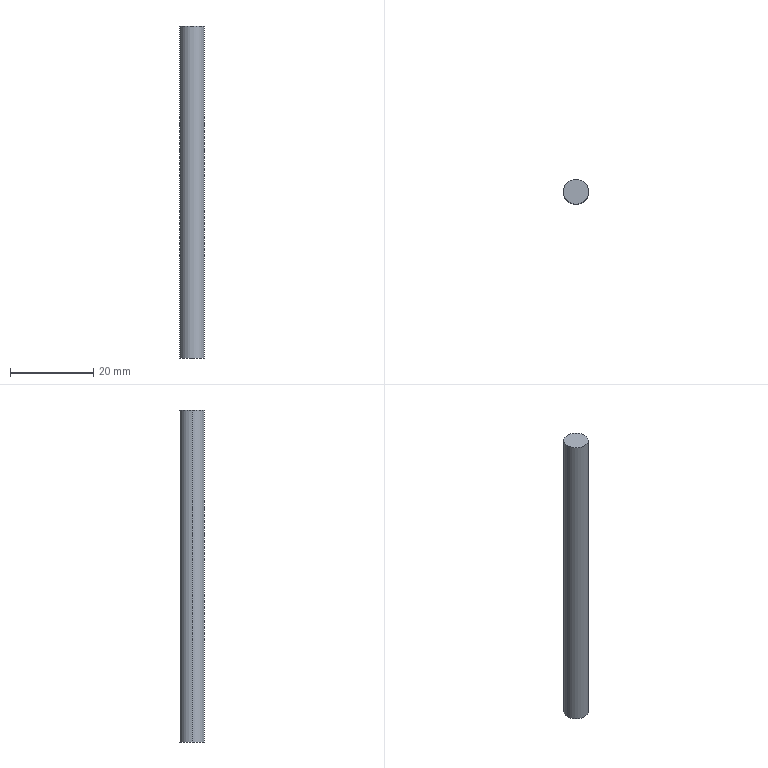Part | SolidWorks | features Extrusion 1 | 1 solid | 4 faces | box 6 x 6 x 80 mm | volume 2262 mm3 | cylinder 2 | plane 2 | commonest cylinder face diameters 6 x2
STEP:
#1=CARTESIAN_POINT('',(3.,0.,80.));
#2=VERTEX_POINT('',#1);
#3=CARTESIAN_POINT('',(-3.,0.,80.));
#4=VERTEX_POINT('',#3);
#5=CARTESIAN_POINT('',(0.,0.,80.));
#6=DIRECTION('',(0.,0.,1.));
#7=DIRECTION('',(1.,0.,0.));
#8=AXIS2_PLACEMENT_3D('',#5,#6,#7);
#9=CIRCLE('',#8,3.);
#10=EDGE_CURVE('',#2,#4,#9,.T.);
#11=ORIENTED_EDGE('',*,*,#10,.F.);
#12=CARTESIAN_POINT('',(3.,0.,0.));
#13=VERTEX_POINT('',#12);
#14=CARTESIAN_POINT('',(3.,0.,80.));
#15=DIRECTION('',(0.,0.,-1.));
#16=VECTOR('',#15,1000.);
#17=LINE('',#14,#16);
#18=EDGE_CURVE('',#2,#13,#17,.T.);
#19=ORIENTED_EDGE('',*,*,#18,.T.);
#20=CARTESIAN_POINT('',(-3.,0.,0.));
#21=VERTEX_POINT('',#20);
#22=CARTESIAN_POINT('',(0.,0.,0.));
#23=DIRECTION('',(0.,0.,1.));
#24=DIRECTION('',(1.,0.,0.));
#25=AXIS2_PLACEMENT_3D('',#22,#23,#24);
#26=CIRCLE('',#25,3.);
#27=EDGE_CURVE('',#13,#21,#26,.T.);
#28=ORIENTED_EDGE('',*,*,#27,.T.);
#29=CARTESIAN_POINT('',(-3.,0.,80.));
#30=DIRECTION('',(0.,0.,-1.));
#31=VECTOR('',#30,1000.);
#32=LINE('',#29,#31);
#33=EDGE_CURVE('',#4,#21,#32,.T.);
#34=ORIENTED_EDGE('',*,*,#33,.F.);
#35=EDGE_LOOP('',(#11,#19,#28,#34));
#36=FACE_OUTER_BOUND('',#35,.T.);
#37=CARTESIAN_POINT('',(0.,0.,80.));
#38=DIRECTION('',(0.,0.,-1.));
#39=DIRECTION('',(-1.,0.,0.));
#40=AXIS2_PLACEMENT_3D('',#37,#38,#39);
#41=CYLINDRICAL_SURFACE('',#40,3.);
#42=ADVANCED_FACE('',(#36),#41,.T.);
#43=ORIENTED_EDGE('',*,*,#18,.F.);
#44=CARTESIAN_POINT('',(0.,0.,80.));
#45=DIRECTION('',(0.,0.,1.));
#46=DIRECTION('',(1.,0.,0.));
#47=AXIS2_PLACEMENT_3D('',#44,#45,#46);
#48=CIRCLE('',#47,3.);
#49=EDGE_CURVE('',#4,#2,#48,.T.);
#50=ORIENTED_EDGE('',*,*,#49,.F.);
#51=ORIENTED_EDGE('',*,*,#33,.T.);
#52=CARTESIAN_POINT('',(0.,0.,0.));
#53=DIRECTION('',(0.,0.,1.));
#54=DIRECTION('',(1.,0.,0.));
#55=AXIS2_PLACEMENT_3D('',#52,#53,#54);
#56=CIRCLE('',#55,3.);
#57=EDGE_CURVE('',#21,#13,#56,.T.);
#58=ORIENTED_EDGE('',*,*,#57,.T.);
#59=EDGE_LOOP('',(#43,#50,#51,#58));
#60=FACE_OUTER_BOUND('',#59,.T.);
#61=CARTESIAN_POINT('',(0.,0.,80.));
#62=DIRECTION('',(0.,0.,-1.));
#63=DIRECTION('',(-1.,0.,0.));
#64=AXIS2_PLACEMENT_3D('',#61,#62,#63);
#65=CYLINDRICAL_SURFACE('',#64,3.);
#66=ADVANCED_FACE('',(#60),#65,.T.);
#67=ORIENTED_EDGE('',*,*,#49,.T.);
#68=ORIENTED_EDGE('',*,*,#10,.T.);
#69=EDGE_LOOP('',(#67,#68));
#70=FACE_OUTER_BOUND('',#69,.T.);
#71=CARTESIAN_POINT('',(0.,0.,80.));
#72=DIRECTION('',(0.,0.,1.));
#73=DIRECTION('',(1.,0.,0.));
#74=AXIS2_PLACEMENT_3D('',#71,#72,#73);
#75=PLANE('',#74);
#76=ADVANCED_FACE('',(#70),#75,.T.);
#77=ORIENTED_EDGE('',*,*,#57,.F.);
#78=ORIENTED_EDGE('',*,*,#27,.F.);
#79=EDGE_LOOP('',(#77,#78));
#80=FACE_OUTER_BOUND('',#79,.T.);
#81=CARTESIAN_POINT('',(0.,0.,0.));
#82=DIRECTION('',(0.,0.,1.));
#83=DIRECTION('',(1.,0.,0.));
#84=AXIS2_PLACEMENT_3D('',#81,#82,#83);
#85=PLANE('',#84);
#86=ADVANCED_FACE('',(#80),#85,.F.);
#87=CLOSED_SHELL('',(#42,#66,#76,#86));
#88=MANIFOLD_SOLID_BREP('',#87);
#89=CARTESIAN_POINT('',(0.,0.,0.));
#90=DIRECTION('',(0.,0.,1.));
#91=DIRECTION('',(1.,0.,0.));
#92=AXIS2_PLACEMENT_3D('',#89,#90,#91);
#93=(LENGTH_UNIT()NAMED_UNIT(*)SI_UNIT(.MILLI.,.METRE.));
#94=UNCERTAINTY_MEASURE_WITH_UNIT(LENGTH_MEASURE(0.00001),#93,'','');
#95=(NAMED_UNIT(*)PLANE_ANGLE_UNIT()SI_UNIT($,.RADIAN.));
#96=(NAMED_UNIT(*)SI_UNIT($,.STERADIAN.)SOLID_ANGLE_UNIT());
#97=(GEOMETRIC_REPRESENTATION_CONTEXT(3)GLOBAL_UNCERTAINTY_ASSIGNED_CONTEXT((#94))GLOBAL_UNIT_ASSIGNED_CONTEXT((#93,#95,#96))REPRESENTATION_CONTEXT('',''));
#98=ADVANCED_BREP_SHAPE_REPRESENTATION('',(#88,#92),#97);